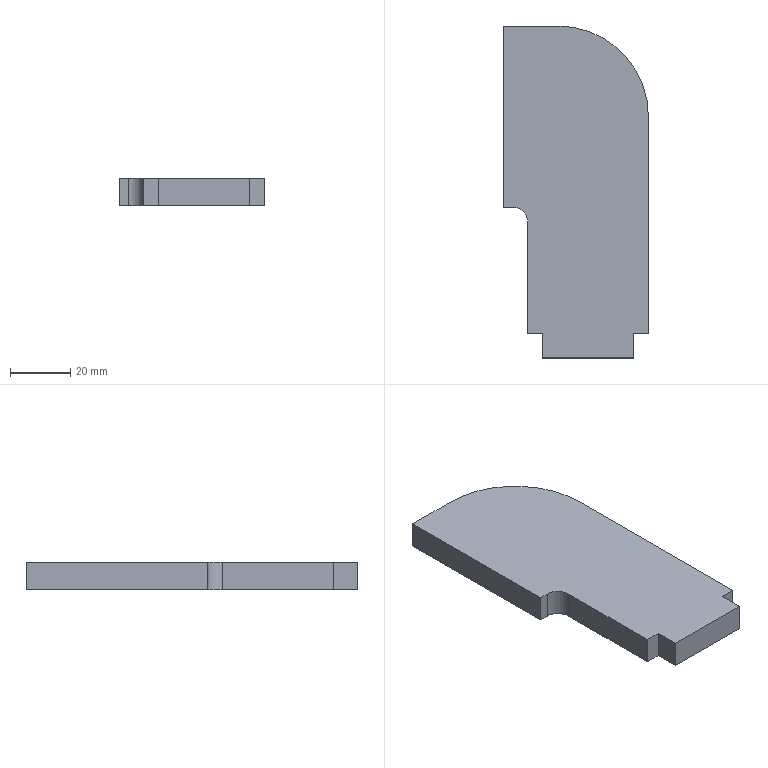Part | SolidWorks | features Fillet 1, FlatPattern 1, SMBaseFlange 1, SheetMetal 1 | 1 solid | 14 faces | box 48 x 110 x 9 mm | volume 41510 mm3 | plane 12 | cylinder 2 | commonest cylinder face diameters 10 x1 60 x1
STEP:
#1=CARTESIAN_POINT('',(0.,80.,0.));
#2=VERTEX_POINT('',#1);
#3=CARTESIAN_POINT('',(-30.,110.,0.));
#4=VERTEX_POINT('',#3);
#5=CARTESIAN_POINT('',(-30.,80.,0.));
#6=DIRECTION('',(0.,0.,1.));
#7=DIRECTION('',(1.,0.,0.));
#8=AXIS2_PLACEMENT_3D('',#5,#6,#7);
#9=CIRCLE('',#8,30.);
#10=EDGE_CURVE('',#2,#4,#9,.T.);
#11=ORIENTED_EDGE('',*,*,#10,.T.);
#12=CARTESIAN_POINT('',(-30.,110.,9.));
#13=VERTEX_POINT('',#12);
#14=CARTESIAN_POINT('',(-30.,110.,9.));
#15=DIRECTION('',(0.,0.,-1.));
#16=VECTOR('',#15,1000.);
#17=LINE('',#14,#16);
#18=EDGE_CURVE('',#13,#4,#17,.T.);
#19=ORIENTED_EDGE('',*,*,#18,.F.);
#20=CARTESIAN_POINT('',(0.,80.,9.));
#21=VERTEX_POINT('',#20);
#22=CARTESIAN_POINT('',(-30.,80.,9.));
#23=DIRECTION('',(0.,0.,1.));
#24=DIRECTION('',(1.,0.,0.));
#25=AXIS2_PLACEMENT_3D('',#22,#23,#24);
#26=CIRCLE('',#25,30.);
#27=EDGE_CURVE('',#21,#13,#26,.T.);
#28=ORIENTED_EDGE('',*,*,#27,.F.);
#29=CARTESIAN_POINT('',(0.,80.,9.));
#30=DIRECTION('',(0.,0.,-1.));
#31=VECTOR('',#30,1000.);
#32=LINE('',#29,#31);
#33=EDGE_CURVE('',#21,#2,#32,.T.);
#34=ORIENTED_EDGE('',*,*,#33,.T.);
#35=EDGE_LOOP('',(#11,#19,#28,#34));
#36=FACE_OUTER_BOUND('',#35,.T.);
#37=CARTESIAN_POINT('',(-30.,80.,9.));
#38=DIRECTION('',(0.,0.,-1.));
#39=DIRECTION('',(-1.,0.,0.));
#40=AXIS2_PLACEMENT_3D('',#37,#38,#39);
#41=CYLINDRICAL_SURFACE('',#40,30.);
#42=ADVANCED_FACE('',(#36),#41,.T.);
#43=CARTESIAN_POINT('',(-48.,110.,0.));
#44=VERTEX_POINT('',#43);
#45=CARTESIAN_POINT('',(-30.,110.,0.));
#46=DIRECTION('',(-1.,0.,0.));
#47=VECTOR('',#46,1000.);
#48=LINE('',#45,#47);
#49=EDGE_CURVE('',#4,#44,#48,.T.);
#50=ORIENTED_EDGE('',*,*,#49,.T.);
#51=CARTESIAN_POINT('',(-48.,110.,9.));
#52=VERTEX_POINT('',#51);
#53=CARTESIAN_POINT('',(-48.,110.,9.));
#54=DIRECTION('',(0.,0.,-1.));
#55=VECTOR('',#54,1000.);
#56=LINE('',#53,#55);
#57=EDGE_CURVE('',#52,#44,#56,.T.);
#58=ORIENTED_EDGE('',*,*,#57,.F.);
#59=CARTESIAN_POINT('',(-30.,110.,9.));
#60=DIRECTION('',(-1.,0.,0.));
#61=VECTOR('',#60,1000.);
#62=LINE('',#59,#61);
#63=EDGE_CURVE('',#13,#52,#62,.T.);
#64=ORIENTED_EDGE('',*,*,#63,.F.);
#65=ORIENTED_EDGE('',*,*,#18,.T.);
#66=EDGE_LOOP('',(#50,#58,#64,#65));
#67=FACE_OUTER_BOUND('',#66,.T.);
#68=CARTESIAN_POINT('',(-30.,110.,9.));
#69=DIRECTION('',(0.,-1.,0.));
#70=DIRECTION('',(0.,0.,-1.));
#71=AXIS2_PLACEMENT_3D('',#68,#69,#70);
#72=PLANE('',#71);
#73=ADVANCED_FACE('',(#67),#72,.F.);
#74=CARTESIAN_POINT('',(-48.,50.,0.));
#75=VERTEX_POINT('',#74);
#76=CARTESIAN_POINT('',(-48.,110.,0.));
#77=DIRECTION('',(0.,-1.,0.));
#78=VECTOR('',#77,1000.);
#79=LINE('',#76,#78);
#80=EDGE_CURVE('',#44,#75,#79,.T.);
#81=ORIENTED_EDGE('',*,*,#80,.T.);
#82=CARTESIAN_POINT('',(-48.,50.,9.));
#83=VERTEX_POINT('',#82);
#84=CARTESIAN_POINT('',(-48.,50.,9.));
#85=DIRECTION('',(0.,0.,-1.));
#86=VECTOR('',#85,1000.);
#87=LINE('',#84,#86);
#88=EDGE_CURVE('',#83,#75,#87,.T.);
#89=ORIENTED_EDGE('',*,*,#88,.F.);
#90=CARTESIAN_POINT('',(-48.,110.,9.));
#91=DIRECTION('',(0.,-1.,0.));
#92=VECTOR('',#91,1000.);
#93=LINE('',#90,#92);
#94=EDGE_CURVE('',#52,#83,#93,.T.);
#95=ORIENTED_EDGE('',*,*,#94,.F.);
#96=ORIENTED_EDGE('',*,*,#57,.T.);
#97=EDGE_LOOP('',(#81,#89,#95,#96));
#98=FACE_OUTER_BOUND('',#97,.T.);
#99=CARTESIAN_POINT('',(-48.,110.,9.));
#100=DIRECTION('',(1.,0.,0.));
#101=DIRECTION('',(0.,0.,-1.));
#102=AXIS2_PLACEMENT_3D('',#99,#100,#101);
#103=PLANE('',#102);
#104=ADVANCED_FACE('',(#98),#103,.F.);
#105=CARTESIAN_POINT('',(-45.,50.,0.));
#106=VERTEX_POINT('',#105);
#107=CARTESIAN_POINT('',(-48.,50.,0.));
#108=DIRECTION('',(1.,0.,0.));
#109=VECTOR('',#108,1000.);
#110=LINE('',#107,#109);
#111=EDGE_CURVE('',#75,#106,#110,.T.);
#112=ORIENTED_EDGE('',*,*,#111,.T.);
#113=CARTESIAN_POINT('',(-45.,50.,9.));
#114=VERTEX_POINT('',#113);
#115=CARTESIAN_POINT('',(-45.,50.,9.));
#116=DIRECTION('',(0.,0.,1.));
#117=VECTOR('',#116,1000.);
#118=LINE('',#115,#117);
#119=EDGE_CURVE('',#106,#114,#118,.T.);
#120=ORIENTED_EDGE('',*,*,#119,.T.);
#121=CARTESIAN_POINT('',(-48.,50.,9.));
#122=DIRECTION('',(1.,0.,0.));
#123=VECTOR('',#122,1000.);
#124=LINE('',#121,#123);
#125=EDGE_CURVE('',#83,#114,#124,.T.);
#126=ORIENTED_EDGE('',*,*,#125,.F.);
#127=ORIENTED_EDGE('',*,*,#88,.T.);
#128=EDGE_LOOP('',(#112,#120,#126,#127));
#129=FACE_OUTER_BOUND('',#128,.T.);
#130=CARTESIAN_POINT('',(-48.,50.,9.));
#131=DIRECTION('',(0.,1.,0.));
#132=DIRECTION('',(-1.,0.,0.));
#133=AXIS2_PLACEMENT_3D('',#130,#131,#132);
#134=PLANE('',#133);
#135=ADVANCED_FACE('',(#129),#134,.F.);
#136=CARTESIAN_POINT('',(-40.,45.,9.));
#137=VERTEX_POINT('',#136);
#138=CARTESIAN_POINT('',(-40.,8.,9.));
#139=VERTEX_POINT('',#138);
#140=CARTESIAN_POINT('',(-40.,50.,9.));
#141=DIRECTION('',(0.,-1.,0.));
#142=VECTOR('',#141,1000.);
#143=LINE('',#140,#142);
#144=EDGE_CURVE('',#137,#139,#143,.T.);
#145=ORIENTED_EDGE('',*,*,#144,.F.);
#146=CARTESIAN_POINT('',(-40.,45.,0.));
#147=VERTEX_POINT('',#146);
#148=CARTESIAN_POINT('',(-40.,45.,0.));
#149=DIRECTION('',(0.,0.,-1.));
#150=VECTOR('',#149,1000.);
#151=LINE('',#148,#150);
#152=EDGE_CURVE('',#137,#147,#151,.T.);
#153=ORIENTED_EDGE('',*,*,#152,.T.);
#154=CARTESIAN_POINT('',(-40.,8.,0.));
#155=VERTEX_POINT('',#154);
#156=CARTESIAN_POINT('',(-40.,50.,0.));
#157=DIRECTION('',(0.,-1.,0.));
#158=VECTOR('',#157,1000.);
#159=LINE('',#156,#158);
#160=EDGE_CURVE('',#147,#155,#159,.T.);
#161=ORIENTED_EDGE('',*,*,#160,.T.);
#162=CARTESIAN_POINT('',(-40.,8.,9.));
#163=DIRECTION('',(0.,0.,-1.));
#164=VECTOR('',#163,1000.);
#165=LINE('',#162,#164);
#166=EDGE_CURVE('',#139,#155,#165,.T.);
#167=ORIENTED_EDGE('',*,*,#166,.F.);
#168=EDGE_LOOP('',(#145,#153,#161,#167));
#169=FACE_OUTER_BOUND('',#168,.T.);
#170=CARTESIAN_POINT('',(-40.,50.,9.));
#171=DIRECTION('',(1.,0.,0.));
#172=DIRECTION('',(0.,1.,0.));
#173=AXIS2_PLACEMENT_3D('',#170,#171,#172);
#174=PLANE('',#173);
#175=ADVANCED_FACE('',(#169),#174,.F.);
#176=CARTESIAN_POINT('',(-35.,8.,0.));
#177=VERTEX_POINT('',#176);
#178=CARTESIAN_POINT('',(-40.,8.,0.));
#179=DIRECTION('',(1.,0.,0.));
#180=VECTOR('',#179,1000.);
#181=LINE('',#178,#180);
#182=EDGE_CURVE('',#155,#177,#181,.T.);
#183=ORIENTED_EDGE('',*,*,#182,.T.);
#184=CARTESIAN_POINT('',(-35.,8.,9.));
#185=VERTEX_POINT('',#184);
#186=CARTESIAN_POINT('',(-35.,8.,9.));
#187=DIRECTION('',(0.,0.,-1.));
#188=VECTOR('',#187,1000.);
#189=LINE('',#186,#188);
#190=EDGE_CURVE('',#185,#177,#189,.T.);
#191=ORIENTED_EDGE('',*,*,#190,.F.);
#192=CARTESIAN_POINT('',(-40.,8.,9.));
#193=DIRECTION('',(1.,0.,0.));
#194=VECTOR('',#193,1000.);
#195=LINE('',#192,#194);
#196=EDGE_CURVE('',#139,#185,#195,.T.);
#197=ORIENTED_EDGE('',*,*,#196,.F.);
#198=ORIENTED_EDGE('',*,*,#166,.T.);
#199=EDGE_LOOP('',(#183,#191,#197,#198));
#200=FACE_OUTER_BOUND('',#199,.T.);
#201=CARTESIAN_POINT('',(-40.,8.,9.));
#202=DIRECTION('',(0.,1.,0.));
#203=DIRECTION('',(-1.,0.,0.));
#204=AXIS2_PLACEMENT_3D('',#201,#202,#203);
#205=PLANE('',#204);
#206=ADVANCED_FACE('',(#200),#205,.F.);
#207=CARTESIAN_POINT('',(-35.,0.,0.));
#208=VERTEX_POINT('',#207);
#209=CARTESIAN_POINT('',(-35.,8.,0.));
#210=DIRECTION('',(0.,-1.,0.));
#211=VECTOR('',#210,1000.);
#212=LINE('',#209,#211);
#213=EDGE_CURVE('',#177,#208,#212,.T.);
#214=ORIENTED_EDGE('',*,*,#213,.T.);
#215=CARTESIAN_POINT('',(-35.,0.,9.));
#216=VERTEX_POINT('',#215);
#217=CARTESIAN_POINT('',(-35.,0.,9.));
#218=DIRECTION('',(0.,0.,-1.));
#219=VECTOR('',#218,1000.);
#220=LINE('',#217,#219);
#221=EDGE_CURVE('',#216,#208,#220,.T.);
#222=ORIENTED_EDGE('',*,*,#221,.F.);
#223=CARTESIAN_POINT('',(-35.,8.,9.));
#224=DIRECTION('',(0.,-1.,0.));
#225=VECTOR('',#224,1000.);
#226=LINE('',#223,#225);
#227=EDGE_CURVE('',#185,#216,#226,.T.);
#228=ORIENTED_EDGE('',*,*,#227,.F.);
#229=ORIENTED_EDGE('',*,*,#190,.T.);
#230=EDGE_LOOP('',(#214,#222,#228,#229));
#231=FACE_OUTER_BOUND('',#230,.T.);
#232=CARTESIAN_POINT('',(-35.,8.,9.));
#233=DIRECTION('',(1.,0.,0.));
#234=DIRECTION('',(0.,0.,-1.));
#235=AXIS2_PLACEMENT_3D('',#232,#233,#234);
#236=PLANE('',#235);
#237=ADVANCED_FACE('',(#231),#236,.F.);
#238=CARTESIAN_POINT('',(-5.,0.,0.));
#239=VERTEX_POINT('',#238);
#240=CARTESIAN_POINT('',(-35.,0.,0.));
#241=DIRECTION('',(1.,0.,0.));
#242=VECTOR('',#241,1000.);
#243=LINE('',#240,#242);
#244=EDGE_CURVE('',#208,#239,#243,.T.);
#245=ORIENTED_EDGE('',*,*,#244,.T.);
#246=CARTESIAN_POINT('',(-5.,0.,9.));
#247=VERTEX_POINT('',#246);
#248=CARTESIAN_POINT('',(-5.,0.,9.));
#249=DIRECTION('',(0.,0.,-1.));
#250=VECTOR('',#249,1000.);
#251=LINE('',#248,#250);
#252=EDGE_CURVE('',#247,#239,#251,.T.);
#253=ORIENTED_EDGE('',*,*,#252,.F.);
#254=CARTESIAN_POINT('',(-35.,0.,9.));
#255=DIRECTION('',(1.,0.,0.));
#256=VECTOR('',#255,1000.);
#257=LINE('',#254,#256);
#258=EDGE_CURVE('',#216,#247,#257,.T.);
#259=ORIENTED_EDGE('',*,*,#258,.F.);
#260=ORIENTED_EDGE('',*,*,#221,.T.);
#261=EDGE_LOOP('',(#245,#253,#259,#260));
#262=FACE_OUTER_BOUND('',#261,.T.);
#263=CARTESIAN_POINT('',(-35.,0.,9.));
#264=DIRECTION('',(0.,1.,0.));
#265=DIRECTION('',(0.,0.,1.));
#266=AXIS2_PLACEMENT_3D('',#263,#264,#265);
#267=PLANE('',#266);
#268=ADVANCED_FACE('',(#262),#267,.F.);
#269=CARTESIAN_POINT('',(-5.,8.,0.));
#270=VERTEX_POINT('',#269);
#271=CARTESIAN_POINT('',(-5.,0.,0.));
#272=DIRECTION('',(0.,1.,0.));
#273=VECTOR('',#272,1000.);
#274=LINE('',#271,#273);
#275=EDGE_CURVE('',#239,#270,#274,.T.);
#276=ORIENTED_EDGE('',*,*,#275,.T.);
#277=CARTESIAN_POINT('',(-5.,8.,9.));
#278=VERTEX_POINT('',#277);
#279=CARTESIAN_POINT('',(-5.,8.,9.));
#280=DIRECTION('',(0.,0.,-1.));
#281=VECTOR('',#280,1000.);
#282=LINE('',#279,#281);
#283=EDGE_CURVE('',#278,#270,#282,.T.);
#284=ORIENTED_EDGE('',*,*,#283,.F.);
#285=CARTESIAN_POINT('',(-5.,0.,9.));
#286=DIRECTION('',(0.,1.,0.));
#287=VECTOR('',#286,1000.);
#288=LINE('',#285,#287);
#289=EDGE_CURVE('',#247,#278,#288,.T.);
#290=ORIENTED_EDGE('',*,*,#289,.F.);
#291=ORIENTED_EDGE('',*,*,#252,.T.);
#292=EDGE_LOOP('',(#276,#284,#290,#291));
#293=FACE_OUTER_BOUND('',#292,.T.);
#294=CARTESIAN_POINT('',(-5.,0.,9.));
#295=DIRECTION('',(-1.,0.,0.));
#296=DIRECTION('',(0.,0.,1.));
#297=AXIS2_PLACEMENT_3D('',#294,#295,#296);
#298=PLANE('',#297);
#299=ADVANCED_FACE('',(#293),#298,.F.);
#300=CARTESIAN_POINT('',(0.,8.,0.));
#301=VERTEX_POINT('',#300);
#302=CARTESIAN_POINT('',(-5.,8.,0.));
#303=DIRECTION('',(1.,0.,0.));
#304=VECTOR('',#303,1000.);
#305=LINE('',#302,#304);
#306=EDGE_CURVE('',#270,#301,#305,.T.);
#307=ORIENTED_EDGE('',*,*,#306,.T.);
#308=CARTESIAN_POINT('',(0.,8.,9.));
#309=VERTEX_POINT('',#308);
#310=CARTESIAN_POINT('',(0.,8.,9.));
#311=DIRECTION('',(0.,0.,-1.));
#312=VECTOR('',#311,1000.);
#313=LINE('',#310,#312);
#314=EDGE_CURVE('',#309,#301,#313,.T.);
#315=ORIENTED_EDGE('',*,*,#314,.F.);
#316=CARTESIAN_POINT('',(-5.,8.,9.));
#317=DIRECTION('',(1.,0.,0.));
#318=VECTOR('',#317,1000.);
#319=LINE('',#316,#318);
#320=EDGE_CURVE('',#278,#309,#319,.T.);
#321=ORIENTED_EDGE('',*,*,#320,.F.);
#322=ORIENTED_EDGE('',*,*,#283,.T.);
#323=EDGE_LOOP('',(#307,#315,#321,#322));
#324=FACE_OUTER_BOUND('',#323,.T.);
#325=CARTESIAN_POINT('',(-5.,8.,9.));
#326=DIRECTION('',(0.,1.,0.));
#327=DIRECTION('',(0.,0.,1.));
#328=AXIS2_PLACEMENT_3D('',#325,#326,#327);
#329=PLANE('',#328);
#330=ADVANCED_FACE('',(#324),#329,.F.);
#331=CARTESIAN_POINT('',(0.,8.,0.));
#332=DIRECTION('',(0.,1.,0.));
#333=VECTOR('',#332,1000.);
#334=LINE('',#331,#333);
#335=EDGE_CURVE('',#301,#2,#334,.T.);
#336=ORIENTED_EDGE('',*,*,#335,.T.);
#337=ORIENTED_EDGE('',*,*,#33,.F.);
#338=CARTESIAN_POINT('',(0.,8.,9.));
#339=DIRECTION('',(0.,1.,0.));
#340=VECTOR('',#339,1000.);
#341=LINE('',#338,#340);
#342=EDGE_CURVE('',#309,#21,#341,.T.);
#343=ORIENTED_EDGE('',*,*,#342,.F.);
#344=ORIENTED_EDGE('',*,*,#314,.T.);
#345=EDGE_LOOP('',(#336,#337,#343,#344));
#346=FACE_OUTER_BOUND('',#345,.T.);
#347=CARTESIAN_POINT('',(0.,8.,9.));
#348=DIRECTION('',(-1.,0.,0.));
#349=DIRECTION('',(0.,0.,1.));
#350=AXIS2_PLACEMENT_3D('',#347,#348,#349);
#351=PLANE('',#350);
#352=ADVANCED_FACE('',(#346),#351,.F.);
#353=ORIENTED_EDGE('',*,*,#27,.T.);
#354=ORIENTED_EDGE('',*,*,#63,.T.);
#355=ORIENTED_EDGE('',*,*,#94,.T.);
#356=ORIENTED_EDGE('',*,*,#125,.T.);
#357=CARTESIAN_POINT('',(-45.,45.,9.));
#358=DIRECTION('',(0.,0.,-1.));
#359=DIRECTION('',(1.,0.,0.));
#360=AXIS2_PLACEMENT_3D('',#357,#358,#359);
#361=CIRCLE('',#360,5.);
#362=EDGE_CURVE('',#114,#137,#361,.T.);
#363=ORIENTED_EDGE('',*,*,#362,.T.);
#364=ORIENTED_EDGE('',*,*,#144,.T.);
#365=ORIENTED_EDGE('',*,*,#196,.T.);
#366=ORIENTED_EDGE('',*,*,#227,.T.);
#367=ORIENTED_EDGE('',*,*,#258,.T.);
#368=ORIENTED_EDGE('',*,*,#289,.T.);
#369=ORIENTED_EDGE('',*,*,#320,.T.);
#370=ORIENTED_EDGE('',*,*,#342,.T.);
#371=EDGE_LOOP('',(#353,#354,#355,#356,#363,#364,#365,#366,#367,#368,#369,#370));
#372=FACE_OUTER_BOUND('',#371,.T.);
#373=CARTESIAN_POINT('',(-30.,80.,9.));
#374=DIRECTION('',(0.,0.,1.));
#375=DIRECTION('',(1.,0.,0.));
#376=AXIS2_PLACEMENT_3D('',#373,#374,#375);
#377=PLANE('',#376);
#378=ADVANCED_FACE('',(#372),#377,.T.);
#379=ORIENTED_EDGE('',*,*,#10,.F.);
#380=ORIENTED_EDGE('',*,*,#335,.F.);
#381=ORIENTED_EDGE('',*,*,#306,.F.);
#382=ORIENTED_EDGE('',*,*,#275,.F.);
#383=ORIENTED_EDGE('',*,*,#244,.F.);
#384=ORIENTED_EDGE('',*,*,#213,.F.);
#385=ORIENTED_EDGE('',*,*,#182,.F.);
#386=ORIENTED_EDGE('',*,*,#160,.F.);
#387=CARTESIAN_POINT('',(-45.,45.,0.));
#388=DIRECTION('',(0.,0.,1.));
#389=DIRECTION('',(1.,0.,0.));
#390=AXIS2_PLACEMENT_3D('',#387,#388,#389);
#391=CIRCLE('',#390,5.);
#392=EDGE_CURVE('',#147,#106,#391,.T.);
#393=ORIENTED_EDGE('',*,*,#392,.T.);
#394=ORIENTED_EDGE('',*,*,#111,.F.);
#395=ORIENTED_EDGE('',*,*,#80,.F.);
#396=ORIENTED_EDGE('',*,*,#49,.F.);
#397=EDGE_LOOP('',(#379,#380,#381,#382,#383,#384,#385,#386,#393,#394,#395,#396));
#398=FACE_OUTER_BOUND('',#397,.T.);
#399=CARTESIAN_POINT('',(-30.,80.,0.));
#400=DIRECTION('',(0.,0.,1.));
#401=DIRECTION('',(1.,0.,0.));
#402=AXIS2_PLACEMENT_3D('',#399,#400,#401);
#403=PLANE('',#402);
#404=ADVANCED_FACE('',(#398),#403,.F.);
#405=ORIENTED_EDGE('',*,*,#362,.F.);
#406=ORIENTED_EDGE('',*,*,#119,.F.);
#407=ORIENTED_EDGE('',*,*,#392,.F.);
#408=ORIENTED_EDGE('',*,*,#152,.F.);
#409=EDGE_LOOP('',(#405,#406,#407,#408));
#410=FACE_OUTER_BOUND('',#409,.T.);
#411=CARTESIAN_POINT('',(-45.,45.,9.));
#412=DIRECTION('',(0.,0.,1.));
#413=DIRECTION('',(1.,0.,0.));
#414=AXIS2_PLACEMENT_3D('',#411,#412,#413);
#415=CYLINDRICAL_SURFACE('',#414,5.);
#416=ADVANCED_FACE('',(#410),#415,.F.);
#417=CLOSED_SHELL('',(#42,#73,#104,#135,#175,#206,#237,#268,#299,#330,#352,#378,#404,#416));
#418=MANIFOLD_SOLID_BREP('',#417);
#419=CARTESIAN_POINT('',(0.,0.,0.));
#420=DIRECTION('',(0.,0.,1.));
#421=DIRECTION('',(1.,0.,0.));
#422=AXIS2_PLACEMENT_3D('',#419,#420,#421);
#423=(LENGTH_UNIT()NAMED_UNIT(*)SI_UNIT(.MILLI.,.METRE.));
#424=UNCERTAINTY_MEASURE_WITH_UNIT(LENGTH_MEASURE(0.00001),#423,'','');
#425=(NAMED_UNIT(*)PLANE_ANGLE_UNIT()SI_UNIT($,.RADIAN.));
#426=(NAMED_UNIT(*)SI_UNIT($,.STERADIAN.)SOLID_ANGLE_UNIT());
#427=(GEOMETRIC_REPRESENTATION_CONTEXT(3)GLOBAL_UNCERTAINTY_ASSIGNED_CONTEXT((#424))GLOBAL_UNIT_ASSIGNED_CONTEXT((#423,#425,#426))REPRESENTATION_CONTEXT('',''));
#428=ADVANCED_BREP_SHAPE_REPRESENTATION('',(#418,#422),#427);